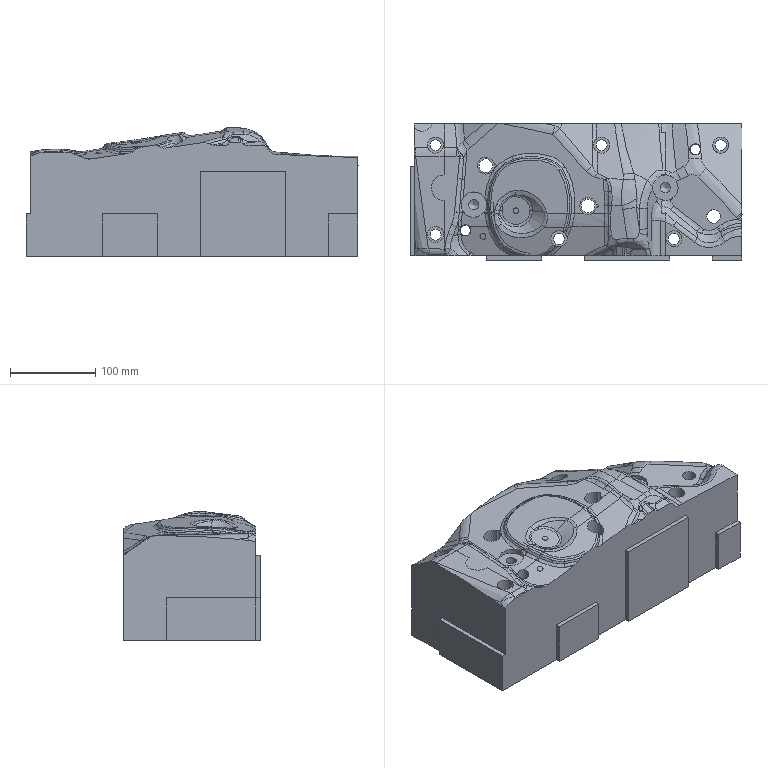Part | NX | features solid 2 | 1 solid | 304 faces | box 393.555 x 160.472 x 151.412 mm | volume 7115826 mm3 | spline 162 | cylinder 77 | plane 61 | sphere 2 | cone 2 | commonest cylinder face diameters 13 x8 10 x7 40 x7 19 x6 20 x6 12 x4